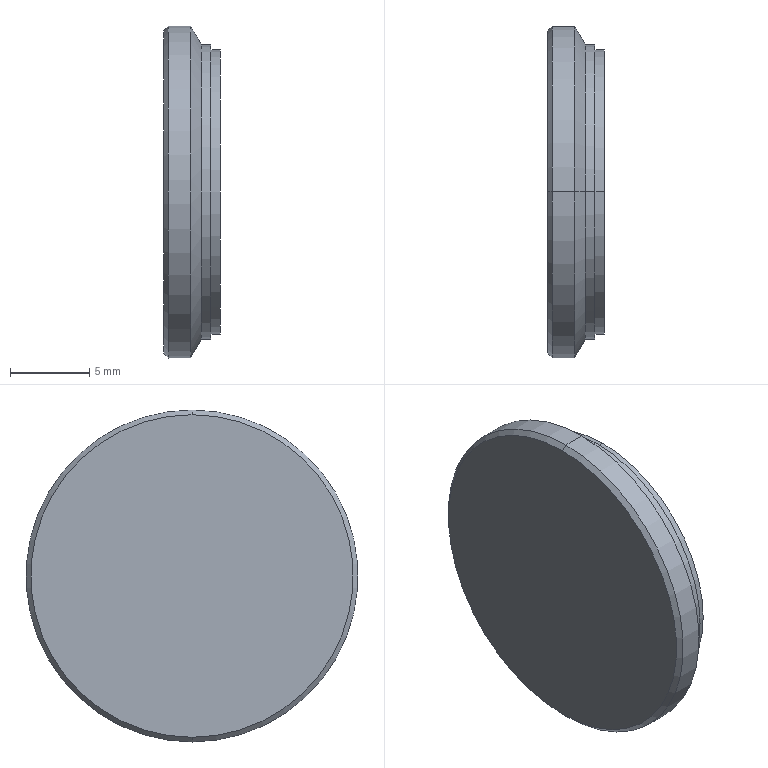Part | STEP file | 2026.6.15-Main Assembly图.sldasm-Part-282 | 1 solid | 13 faces | box 3.6 x 21 x 21 mm | volume 1117 mm3 | cylinder 6 | cone 4 | plane 3 | commonest cylinder face diameters 17.97 x2 18.6 x2 21 x2
STEP:
#1=CARTESIAN_POINT('',(-1618.188,1424.264,3417.071));
#2=VERTEX_POINT('',#1);
#3=CARTESIAN_POINT('',(-1618.188,1424.264,3399.101));
#4=VERTEX_POINT('',#3);
#5=CARTESIAN_POINT('',(-1618.188,1424.264,3408.086));
#6=DIRECTION('',(-1.,0.,0.));
#7=DIRECTION('',(0.,0.,1.));
#8=AXIS2_PLACEMENT_3D('',#5,#6,#7);
#9=CIRCLE('',#8,8.985);
#10=EDGE_CURVE('',#2,#4,#9,.T.);
#11=ORIENTED_EDGE('',*,*,#10,.F.);
#12=CARTESIAN_POINT('',(-1618.188,1424.264,3408.086));
#13=DIRECTION('',(-1.,0.,0.));
#14=DIRECTION('',(0.,0.,1.));
#15=AXIS2_PLACEMENT_3D('',#12,#13,#14);
#16=CIRCLE('',#15,8.985);
#17=EDGE_CURVE('',#4,#2,#16,.T.);
#18=ORIENTED_EDGE('',*,*,#17,.F.);
#19=EDGE_LOOP('',(#11,#18));
#20=FACE_OUTER_BOUND('',#19,.T.);
#21=CARTESIAN_POINT('',(-1618.188,1424.264,3408.086));
#22=DIRECTION('',(-1.,0.,0.));
#23=DIRECTION('',(0.,0.,1.));
#24=AXIS2_PLACEMENT_3D('',#21,#22,#23);
#25=PLANE('',#24);
#26=ADVANCED_FACE('',(#20),#25,.F.);
#27=CARTESIAN_POINT('',(-1618.788,1424.264,3399.101));
#28=VERTEX_POINT('',#27);
#29=CARTESIAN_POINT('',(-1618.788,1424.264,3399.101));
#30=DIRECTION('',(1.,0.,0.));
#31=VECTOR('',#30,1000.);
#32=LINE('',#29,#31);
#33=EDGE_CURVE('',#28,#4,#32,.T.);
#34=ORIENTED_EDGE('',*,*,#33,.T.);
#35=ORIENTED_EDGE('',*,*,#17,.T.);
#36=CARTESIAN_POINT('',(-1618.788,1424.264,3417.071));
#37=VERTEX_POINT('',#36);
#38=CARTESIAN_POINT('',(-1618.788,1424.264,3417.071));
#39=DIRECTION('',(1.,0.,0.));
#40=VECTOR('',#39,1000.);
#41=LINE('',#38,#40);
#42=EDGE_CURVE('',#37,#2,#41,.T.);
#43=ORIENTED_EDGE('',*,*,#42,.F.);
#44=CARTESIAN_POINT('',(-1618.788,1424.264,3408.086));
#45=DIRECTION('',(-1.,0.,0.));
#46=DIRECTION('',(0.,0.,1.));
#47=AXIS2_PLACEMENT_3D('',#44,#45,#46);
#48=CIRCLE('',#47,8.985);
#49=EDGE_CURVE('',#28,#37,#48,.T.);
#50=ORIENTED_EDGE('',*,*,#49,.F.);
#51=EDGE_LOOP('',(#34,#35,#43,#50));
#52=FACE_OUTER_BOUND('',#51,.T.);
#53=CARTESIAN_POINT('',(-1618.788,1424.264,3408.086));
#54=DIRECTION('',(-1.,0.,0.));
#55=DIRECTION('',(0.,0.,-1.));
#56=AXIS2_PLACEMENT_3D('',#53,#54,#55);
#57=CYLINDRICAL_SURFACE('',#56,8.985);
#58=ADVANCED_FACE('',(#52),#57,.T.);
#59=CARTESIAN_POINT('',(-1618.788,1424.264,3417.386));
#60=VERTEX_POINT('',#59);
#61=CARTESIAN_POINT('',(-1618.788,1424.264,3398.786));
#62=VERTEX_POINT('',#61);
#63=CARTESIAN_POINT('',(-1618.788,1424.264,3408.086));
#64=DIRECTION('',(-1.,0.,0.));
#65=DIRECTION('',(0.,0.,1.));
#66=AXIS2_PLACEMENT_3D('',#63,#64,#65);
#67=CIRCLE('',#66,9.3);
#68=EDGE_CURVE('',#60,#62,#67,.T.);
#69=ORIENTED_EDGE('',*,*,#68,.F.);
#70=CARTESIAN_POINT('',(-1618.788,1424.264,3408.086));
#71=DIRECTION('',(-1.,0.,0.));
#72=DIRECTION('',(0.,0.,1.));
#73=AXIS2_PLACEMENT_3D('',#70,#71,#72);
#74=CIRCLE('',#73,9.3);
#75=EDGE_CURVE('',#62,#60,#74,.T.);
#76=ORIENTED_EDGE('',*,*,#75,.F.);
#77=EDGE_LOOP('',(#69,#76));
#78=FACE_OUTER_BOUND('',#77,.T.);
#79=CARTESIAN_POINT('',(-1618.788,1424.264,3408.086));
#80=DIRECTION('',(-1.,0.,0.));
#81=DIRECTION('',(0.,0.,1.));
#82=AXIS2_PLACEMENT_3D('',#79,#80,#81);
#83=CIRCLE('',#82,8.985);
#84=EDGE_CURVE('',#37,#28,#83,.T.);
#85=ORIENTED_EDGE('',*,*,#84,.T.);
#86=ORIENTED_EDGE('',*,*,#49,.T.);
#87=EDGE_LOOP('',(#85,#86));
#88=FACE_BOUND('',#87,.T.);
#89=CARTESIAN_POINT('',(-1618.788,1428.743,3408.096));
#90=DIRECTION('',(1.,0.,0.));
#91=DIRECTION('',(0.,0.,1.));
#92=AXIS2_PLACEMENT_3D('',#89,#90,#91);
#93=PLANE('',#92);
#94=ADVANCED_FACE('',(#78,#88),#93,.T.);
#95=CARTESIAN_POINT('',(-1619.388,1424.264,3398.786));
#96=VERTEX_POINT('',#95);
#97=CARTESIAN_POINT('',(-1619.388,1424.264,3398.786));
#98=DIRECTION('',(1.,0.,0.));
#99=VECTOR('',#98,1000.);
#100=LINE('',#97,#99);
#101=EDGE_CURVE('',#96,#62,#100,.T.);
#102=ORIENTED_EDGE('',*,*,#101,.T.);
#103=ORIENTED_EDGE('',*,*,#75,.T.);
#104=CARTESIAN_POINT('',(-1619.388,1424.264,3417.386));
#105=VERTEX_POINT('',#104);
#106=CARTESIAN_POINT('',(-1619.388,1424.264,3417.386));
#107=DIRECTION('',(1.,0.,0.));
#108=VECTOR('',#107,1000.);
#109=LINE('',#106,#108);
#110=EDGE_CURVE('',#105,#60,#109,.T.);
#111=ORIENTED_EDGE('',*,*,#110,.F.);
#112=CARTESIAN_POINT('',(-1619.388,1424.264,3408.086));
#113=DIRECTION('',(-1.,0.,0.));
#114=DIRECTION('',(0.,0.,1.));
#115=AXIS2_PLACEMENT_3D('',#112,#113,#114);
#116=CIRCLE('',#115,9.3);
#117=EDGE_CURVE('',#96,#105,#116,.T.);
#118=ORIENTED_EDGE('',*,*,#117,.F.);
#119=EDGE_LOOP('',(#102,#103,#111,#118));
#120=FACE_OUTER_BOUND('',#119,.T.);
#121=CARTESIAN_POINT('',(-1619.388,1424.264,3408.086));
#122=DIRECTION('',(-1.,0.,0.));
#123=DIRECTION('',(0.,0.,-1.));
#124=AXIS2_PLACEMENT_3D('',#121,#122,#123);
#125=CYLINDRICAL_SURFACE('',#124,9.3);
#126=ADVANCED_FACE('',(#120),#125,.T.);
#127=CARTESIAN_POINT('',(-1620.081,1424.264,3397.586));
#128=VERTEX_POINT('',#127);
#129=CARTESIAN_POINT('',(-1620.081,1424.264,3397.586));
#130=DIRECTION('',(0.5,0.,0.866));
#131=VECTOR('',#130,1000.);
#132=LINE('',#129,#131);
#133=EDGE_CURVE('',#128,#96,#132,.T.);
#134=ORIENTED_EDGE('',*,*,#133,.T.);
#135=ORIENTED_EDGE('',*,*,#117,.T.);
#136=CARTESIAN_POINT('',(-1620.081,1424.264,3418.586));
#137=VERTEX_POINT('',#136);
#138=CARTESIAN_POINT('',(-1620.081,1424.264,3418.586));
#139=DIRECTION('',(0.5,0.,-0.866));
#140=VECTOR('',#139,1000.);
#141=LINE('',#138,#140);
#142=EDGE_CURVE('',#137,#105,#141,.T.);
#143=ORIENTED_EDGE('',*,*,#142,.F.);
#144=CARTESIAN_POINT('',(-1620.081,1424.264,3408.086));
#145=DIRECTION('',(-1.,0.,0.));
#146=DIRECTION('',(0.,0.,1.));
#147=AXIS2_PLACEMENT_3D('',#144,#145,#146);
#148=CIRCLE('',#147,10.5);
#149=EDGE_CURVE('',#128,#137,#148,.T.);
#150=ORIENTED_EDGE('',*,*,#149,.F.);
#151=EDGE_LOOP('',(#134,#135,#143,#150));
#152=FACE_OUTER_BOUND('',#151,.T.);
#153=CARTESIAN_POINT('',(-1620.081,1424.264,3408.086));
#154=DIRECTION('',(-1.,0.,0.));
#155=DIRECTION('',(0.,0.,-1.));
#156=AXIS2_PLACEMENT_3D('',#153,#154,#155);
#157=CONICAL_SURFACE('',#156,10.5,1.047);
#158=ADVANCED_FACE('',(#152),#157,.T.);
#159=CARTESIAN_POINT('',(-1621.488,1424.264,3397.586));
#160=VERTEX_POINT('',#159);
#161=CARTESIAN_POINT('',(-1621.788,1424.264,3397.586));
#162=DIRECTION('',(1.,0.,0.));
#163=VECTOR('',#162,1000.);
#164=LINE('',#161,#163);
#165=EDGE_CURVE('',#160,#128,#164,.T.);
#166=ORIENTED_EDGE('',*,*,#165,.T.);
#167=ORIENTED_EDGE('',*,*,#149,.T.);
#168=CARTESIAN_POINT('',(-1621.488,1424.264,3418.586));
#169=VERTEX_POINT('',#168);
#170=CARTESIAN_POINT('',(-1621.788,1424.264,3418.586));
#171=DIRECTION('',(1.,0.,0.));
#172=VECTOR('',#171,1000.);
#173=LINE('',#170,#172);
#174=EDGE_CURVE('',#169,#137,#173,.T.);
#175=ORIENTED_EDGE('',*,*,#174,.F.);
#176=CARTESIAN_POINT('',(-1621.488,1424.264,3408.086));
#177=DIRECTION('',(-1.,0.,0.));
#178=DIRECTION('',(0.,0.,-1.));
#179=AXIS2_PLACEMENT_3D('',#176,#177,#178);
#180=CIRCLE('',#179,10.5);
#181=EDGE_CURVE('',#160,#169,#180,.T.);
#182=ORIENTED_EDGE('',*,*,#181,.F.);
#183=EDGE_LOOP('',(#166,#167,#175,#182));
#184=FACE_OUTER_BOUND('',#183,.T.);
#185=CARTESIAN_POINT('',(-1621.788,1424.264,3408.086));
#186=DIRECTION('',(-1.,0.,0.));
#187=DIRECTION('',(0.,0.,-1.));
#188=AXIS2_PLACEMENT_3D('',#185,#186,#187);
#189=CYLINDRICAL_SURFACE('',#188,10.5);
#190=ADVANCED_FACE('',(#184),#189,.T.);
#191=CARTESIAN_POINT('',(-1621.788,1424.264,3418.286));
#192=VERTEX_POINT('',#191);
#193=CARTESIAN_POINT('',(-1621.488,1424.264,3418.586));
#194=DIRECTION('',(0.7071,0.,0.7071));
#195=VECTOR('',#194,1000.);
#196=LINE('',#193,#195);
#197=EDGE_CURVE('',#192,#169,#196,.T.);
#198=ORIENTED_EDGE('',*,*,#197,.F.);
#199=CARTESIAN_POINT('',(-1621.788,1424.264,3397.886));
#200=VERTEX_POINT('',#199);
#201=CARTESIAN_POINT('',(-1621.788,1424.264,3408.086));
#202=DIRECTION('',(-1.,0.,0.));
#203=DIRECTION('',(0.,0.,-1.));
#204=AXIS2_PLACEMENT_3D('',#201,#202,#203);
#205=CIRCLE('',#204,10.2);
#206=EDGE_CURVE('',#200,#192,#205,.T.);
#207=ORIENTED_EDGE('',*,*,#206,.F.);
#208=CARTESIAN_POINT('',(-1621.488,1424.264,3397.586));
#209=DIRECTION('',(0.7071,0.,-0.7071));
#210=VECTOR('',#209,1000.);
#211=LINE('',#208,#210);
#212=EDGE_CURVE('',#200,#160,#211,.T.);
#213=ORIENTED_EDGE('',*,*,#212,.T.);
#214=ORIENTED_EDGE('',*,*,#181,.T.);
#215=EDGE_LOOP('',(#198,#207,#213,#214));
#216=FACE_OUTER_BOUND('',#215,.T.);
#217=CARTESIAN_POINT('',(-1621.488,1424.264,3408.086));
#218=DIRECTION('',(1.,0.,0.));
#219=DIRECTION('',(0.,0.,1.));
#220=AXIS2_PLACEMENT_3D('',#217,#218,#219);
#221=CONICAL_SURFACE('',#220,10.5,0.7854);
#222=ADVANCED_FACE('',(#216),#221,.T.);
#223=ORIENTED_EDGE('',*,*,#206,.T.);
#224=CARTESIAN_POINT('',(-1621.788,1424.264,3408.086));
#225=DIRECTION('',(-1.,0.,0.));
#226=DIRECTION('',(0.,0.,-1.));
#227=AXIS2_PLACEMENT_3D('',#224,#225,#226);
#228=CIRCLE('',#227,10.2);
#229=EDGE_CURVE('',#192,#200,#228,.T.);
#230=ORIENTED_EDGE('',*,*,#229,.T.);
#231=EDGE_LOOP('',(#223,#230));
#232=FACE_OUTER_BOUND('',#231,.T.);
#233=CARTESIAN_POINT('',(-1621.788,1424.264,3408.086));
#234=DIRECTION('',(-1.,0.,0.));
#235=DIRECTION('',(0.,0.,1.));
#236=AXIS2_PLACEMENT_3D('',#233,#234,#235);
#237=PLANE('',#236);
#238=ADVANCED_FACE('',(#232),#237,.T.);
#239=ORIENTED_EDGE('',*,*,#10,.T.);
#240=ORIENTED_EDGE('',*,*,#33,.F.);
#241=ORIENTED_EDGE('',*,*,#84,.F.);
#242=ORIENTED_EDGE('',*,*,#42,.T.);
#243=EDGE_LOOP('',(#239,#240,#241,#242));
#244=FACE_OUTER_BOUND('',#243,.T.);
#245=CARTESIAN_POINT('',(-1618.788,1424.264,3408.086));
#246=DIRECTION('',(-1.,0.,0.));
#247=DIRECTION('',(0.,0.,-1.));
#248=AXIS2_PLACEMENT_3D('',#245,#246,#247);
#249=CYLINDRICAL_SURFACE('',#248,8.985);
#250=ADVANCED_FACE('',(#244),#249,.T.);
#251=ORIENTED_EDGE('',*,*,#68,.T.);
#252=ORIENTED_EDGE('',*,*,#101,.F.);
#253=CARTESIAN_POINT('',(-1619.388,1424.264,3408.086));
#254=DIRECTION('',(-1.,0.,0.));
#255=DIRECTION('',(0.,0.,1.));
#256=AXIS2_PLACEMENT_3D('',#253,#254,#255);
#257=CIRCLE('',#256,9.3);
#258=EDGE_CURVE('',#105,#96,#257,.T.);
#259=ORIENTED_EDGE('',*,*,#258,.F.);
#260=ORIENTED_EDGE('',*,*,#110,.T.);
#261=EDGE_LOOP('',(#251,#252,#259,#260));
#262=FACE_OUTER_BOUND('',#261,.T.);
#263=CARTESIAN_POINT('',(-1619.388,1424.264,3408.086));
#264=DIRECTION('',(-1.,0.,0.));
#265=DIRECTION('',(0.,0.,-1.));
#266=AXIS2_PLACEMENT_3D('',#263,#264,#265);
#267=CYLINDRICAL_SURFACE('',#266,9.3);
#268=ADVANCED_FACE('',(#262),#267,.T.);
#269=ORIENTED_EDGE('',*,*,#258,.T.);
#270=ORIENTED_EDGE('',*,*,#133,.F.);
#271=CARTESIAN_POINT('',(-1620.081,1424.264,3408.086));
#272=DIRECTION('',(-1.,0.,0.));
#273=DIRECTION('',(0.,0.,1.));
#274=AXIS2_PLACEMENT_3D('',#271,#272,#273);
#275=CIRCLE('',#274,10.5);
#276=EDGE_CURVE('',#137,#128,#275,.T.);
#277=ORIENTED_EDGE('',*,*,#276,.F.);
#278=ORIENTED_EDGE('',*,*,#142,.T.);
#279=EDGE_LOOP('',(#269,#270,#277,#278));
#280=FACE_OUTER_BOUND('',#279,.T.);
#281=CARTESIAN_POINT('',(-1620.081,1424.264,3408.086));
#282=DIRECTION('',(-1.,0.,0.));
#283=DIRECTION('',(0.,0.,-1.));
#284=AXIS2_PLACEMENT_3D('',#281,#282,#283);
#285=CONICAL_SURFACE('',#284,10.5,1.047);
#286=ADVANCED_FACE('',(#280),#285,.T.);
#287=ORIENTED_EDGE('',*,*,#276,.T.);
#288=ORIENTED_EDGE('',*,*,#165,.F.);
#289=CARTESIAN_POINT('',(-1621.488,1424.264,3408.086));
#290=DIRECTION('',(-1.,0.,0.));
#291=DIRECTION('',(0.,0.,-1.));
#292=AXIS2_PLACEMENT_3D('',#289,#290,#291);
#293=CIRCLE('',#292,10.5);
#294=EDGE_CURVE('',#169,#160,#293,.T.);
#295=ORIENTED_EDGE('',*,*,#294,.F.);
#296=ORIENTED_EDGE('',*,*,#174,.T.);
#297=EDGE_LOOP('',(#287,#288,#295,#296));
#298=FACE_OUTER_BOUND('',#297,.T.);
#299=CARTESIAN_POINT('',(-1621.788,1424.264,3408.086));
#300=DIRECTION('',(-1.,0.,0.));
#301=DIRECTION('',(0.,0.,-1.));
#302=AXIS2_PLACEMENT_3D('',#299,#300,#301);
#303=CYLINDRICAL_SURFACE('',#302,10.5);
#304=ADVANCED_FACE('',(#298),#303,.T.);
#305=ORIENTED_EDGE('',*,*,#229,.F.);
#306=ORIENTED_EDGE('',*,*,#197,.T.);
#307=ORIENTED_EDGE('',*,*,#294,.T.);
#308=ORIENTED_EDGE('',*,*,#212,.F.);
#309=EDGE_LOOP('',(#305,#306,#307,#308));
#310=FACE_OUTER_BOUND('',#309,.T.);
#311=CARTESIAN_POINT('',(-1621.488,1424.264,3408.086));
#312=DIRECTION('',(1.,0.,0.));
#313=DIRECTION('',(0.,0.,1.));
#314=AXIS2_PLACEMENT_3D('',#311,#312,#313);
#315=CONICAL_SURFACE('',#314,10.5,0.7854);
#316=ADVANCED_FACE('',(#310),#315,.T.);
#317=CLOSED_SHELL('',(#26,#58,#94,#126,#158,#190,#222,#238,#250,#268,#286,#304,#316));
#318=MANIFOLD_SOLID_BREP('',#317);
#319=CARTESIAN_POINT('',(0.,0.,0.));
#320=DIRECTION('',(0.,0.,1.));
#321=DIRECTION('',(1.,0.,0.));
#322=AXIS2_PLACEMENT_3D('',#319,#320,#321);
#323=(LENGTH_UNIT()NAMED_UNIT(*)SI_UNIT(.MILLI.,.METRE.));
#324=UNCERTAINTY_MEASURE_WITH_UNIT(LENGTH_MEASURE(0.00001),#323,'','');
#325=(NAMED_UNIT(*)PLANE_ANGLE_UNIT()SI_UNIT($,.RADIAN.));
#326=(NAMED_UNIT(*)SI_UNIT($,.STERADIAN.)SOLID_ANGLE_UNIT());
#327=(GEOMETRIC_REPRESENTATION_CONTEXT(3)GLOBAL_UNCERTAINTY_ASSIGNED_CONTEXT((#324))GLOBAL_UNIT_ASSIGNED_CONTEXT((#323,#325,#326))REPRESENTATION_CONTEXT('',''));
#328=ADVANCED_BREP_SHAPE_REPRESENTATION('',(#318,#322),#327);